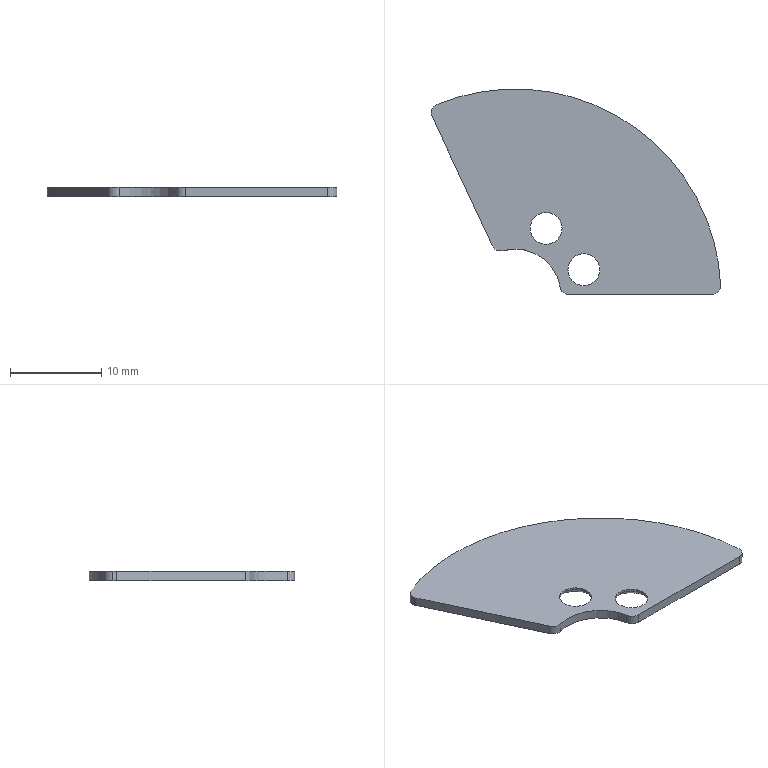Part | NX | features BREP 1 | 1 solid | 19 faces | box 31.647 x 22.5 x 1 mm | volume 455.867 mm3 | cylinder 11 | cone 4 | plane 4 | commonest cylinder face diameters 2 x5 3.5 x4 10 x1 45 x1
STEP:
#1=CARTESIAN_POINT('',(-2.5,5.362,1.));
#2=VERTEX_POINT('',#1);
#3=CARTESIAN_POINT('',(-1.328,4.82,1.));
#4=VERTEX_POINT('',#3);
#5=CARTESIAN_POINT('',(-1.594,5.784,1.));
#6=DIRECTION('',(0.,0.,1.));
#7=DIRECTION('',(1.,0.,0.));
#8=AXIS2_PLACEMENT_3D('',#5,#6,#7);
#9=CIRCLE('',#8,1.);
#10=EDGE_CURVE('',#2,#4,#9,.T.);
#11=ORIENTED_EDGE('',*,*,#10,.F.);
#12=CARTESIAN_POINT('',(-2.5,5.362,0.));
#13=VERTEX_POINT('',#12);
#14=CARTESIAN_POINT('',(-2.5,5.362,10.));
#15=DIRECTION('',(0.,0.,1.));
#16=VECTOR('',#15,1000.);
#17=LINE('',#14,#16);
#18=EDGE_CURVE('',#13,#2,#17,.T.);
#19=ORIENTED_EDGE('',*,*,#18,.F.);
#20=CARTESIAN_POINT('',(-1.328,4.82,0.));
#21=VERTEX_POINT('',#20);
#22=CARTESIAN_POINT('',(-1.594,5.784,0.));
#23=DIRECTION('',(0.,0.,-1.));
#24=DIRECTION('',(1.,0.,0.));
#25=AXIS2_PLACEMENT_3D('',#22,#23,#24);
#26=CIRCLE('',#25,1.);
#27=EDGE_CURVE('',#21,#13,#26,.T.);
#28=ORIENTED_EDGE('',*,*,#27,.F.);
#29=CARTESIAN_POINT('',(-1.328,4.82,1.));
#30=DIRECTION('',(0.,0.,-1.));
#31=VECTOR('',#30,1000.);
#32=LINE('',#29,#31);
#33=EDGE_CURVE('',#4,#21,#32,.T.);
#34=ORIENTED_EDGE('',*,*,#33,.F.);
#35=EDGE_LOOP('',(#11,#19,#28,#34));
#36=FACE_BOUND('',#35,.T.);
#37=CARTESIAN_POINT('',(-1.594,5.784,1.));
#38=DIRECTION('',(0.,0.,-1.));
#39=DIRECTION('',(-1.,0.,0.));
#40=AXIS2_PLACEMENT_3D('',#37,#38,#39);
#41=CYLINDRICAL_SURFACE('',#40,1.);
#42=ADVANCED_FACE('',(#36),#41,.T.);
#43=CARTESIAN_POINT('',(5.916,0.,0.));
#44=VERTEX_POINT('',#43);
#45=CARTESIAN_POINT('',(4.93,0.8333,0.));
#46=VERTEX_POINT('',#45);
#47=CARTESIAN_POINT('',(5.916,1.,0.));
#48=DIRECTION('',(0.,0.,-1.));
#49=DIRECTION('',(1.,0.,0.));
#50=AXIS2_PLACEMENT_3D('',#47,#48,#49);
#51=CIRCLE('',#50,1.);
#52=EDGE_CURVE('',#44,#46,#51,.T.);
#53=ORIENTED_EDGE('',*,*,#52,.F.);
#54=CARTESIAN_POINT('',(5.916,0.,1.));
#55=VERTEX_POINT('',#54);
#56=CARTESIAN_POINT('',(5.916,0.,10.));
#57=DIRECTION('',(0.,0.,-1.));
#58=VECTOR('',#57,1000.);
#59=LINE('',#56,#58);
#60=EDGE_CURVE('',#55,#44,#59,.T.);
#61=ORIENTED_EDGE('',*,*,#60,.F.);
#62=CARTESIAN_POINT('',(4.93,0.8333,1.));
#63=VERTEX_POINT('',#62);
#64=CARTESIAN_POINT('',(5.916,1.,1.));
#65=DIRECTION('',(0.,0.,1.));
#66=DIRECTION('',(1.,0.,0.));
#67=AXIS2_PLACEMENT_3D('',#64,#65,#66);
#68=CIRCLE('',#67,1.);
#69=EDGE_CURVE('',#63,#55,#68,.T.);
#70=ORIENTED_EDGE('',*,*,#69,.F.);
#71=CARTESIAN_POINT('',(4.93,0.8333,1.));
#72=DIRECTION('',(0.,0.,1.));
#73=VECTOR('',#72,1000.);
#74=LINE('',#71,#73);
#75=EDGE_CURVE('',#46,#63,#74,.T.);
#76=ORIENTED_EDGE('',*,*,#75,.F.);
#77=EDGE_LOOP('',(#53,#61,#70,#76));
#78=FACE_BOUND('',#77,.T.);
#79=CARTESIAN_POINT('',(5.916,1.,1.));
#80=DIRECTION('',(0.,0.,-1.));
#81=DIRECTION('',(-1.,0.,0.));
#82=AXIS2_PLACEMENT_3D('',#79,#80,#81);
#83=CYLINDRICAL_SURFACE('',#82,1.);
#84=ADVANCED_FACE('',(#78),#83,.T.);
#85=CARTESIAN_POINT('',(-9.17,19.887,1.));
#86=VERTEX_POINT('',#85);
#87=CARTESIAN_POINT('',(-9.17,19.887,0.));
#88=VERTEX_POINT('',#87);
#89=CARTESIAN_POINT('',(-9.17,19.887,1.));
#90=DIRECTION('',(0.,0.,-1.));
#91=VECTOR('',#90,1000.);
#92=LINE('',#89,#91);
#93=EDGE_CURVE('',#86,#88,#92,.T.);
#94=ORIENTED_EDGE('',*,*,#93,.F.);
#95=CARTESIAN_POINT('',(-8.55,20.812,1.));
#96=VERTEX_POINT('',#95);
#97=CARTESIAN_POINT('',(-8.17,19.887,1.));
#98=DIRECTION('',(0.,0.,1.));
#99=DIRECTION('',(1.,0.,0.));
#100=AXIS2_PLACEMENT_3D('',#97,#98,#99);
#101=CIRCLE('',#100,1.);
#102=EDGE_CURVE('',#96,#86,#101,.T.);
#103=ORIENTED_EDGE('',*,*,#102,.F.);
#104=CARTESIAN_POINT('',(-8.55,20.812,0.));
#105=VERTEX_POINT('',#104);
#106=CARTESIAN_POINT('',(-8.55,20.812,1.));
#107=DIRECTION('',(0.,0.,1.));
#108=VECTOR('',#107,1000.);
#109=LINE('',#106,#108);
#110=EDGE_CURVE('',#105,#96,#109,.T.);
#111=ORIENTED_EDGE('',*,*,#110,.F.);
#112=CARTESIAN_POINT('',(-8.17,19.887,0.));
#113=DIRECTION('',(0.,0.,-1.));
#114=DIRECTION('',(1.,0.,0.));
#115=AXIS2_PLACEMENT_3D('',#112,#113,#114);
#116=CIRCLE('',#115,1.);
#117=EDGE_CURVE('',#88,#105,#116,.T.);
#118=ORIENTED_EDGE('',*,*,#117,.F.);
#119=EDGE_LOOP('',(#94,#103,#111,#118));
#120=FACE_BOUND('',#119,.T.);
#121=CARTESIAN_POINT('',(-8.17,19.887,1.));
#122=DIRECTION('',(0.,0.,-1.));
#123=DIRECTION('',(-1.,0.,0.));
#124=AXIS2_PLACEMENT_3D('',#121,#122,#123);
#125=CYLINDRICAL_SURFACE('',#124,1.);
#126=ADVANCED_FACE('',(#120),#125,.T.);
#127=CARTESIAN_POINT('',(22.476,1.047,0.));
#128=VERTEX_POINT('',#127);
#129=CARTESIAN_POINT('',(21.477,0.,0.));
#130=VERTEX_POINT('',#129);
#131=CARTESIAN_POINT('',(21.477,1.,0.));
#132=DIRECTION('',(0.,0.,-1.));
#133=DIRECTION('',(1.,0.,0.));
#134=AXIS2_PLACEMENT_3D('',#131,#132,#133);
#135=CIRCLE('',#134,1.);
#136=EDGE_CURVE('',#128,#130,#135,.T.);
#137=ORIENTED_EDGE('',*,*,#136,.F.);
#138=CARTESIAN_POINT('',(22.476,1.047,1.));
#139=VERTEX_POINT('',#138);
#140=CARTESIAN_POINT('',(22.476,1.047,1.));
#141=DIRECTION('',(0.,0.,-1.));
#142=VECTOR('',#141,1000.);
#143=LINE('',#140,#142);
#144=EDGE_CURVE('',#139,#128,#143,.T.);
#145=ORIENTED_EDGE('',*,*,#144,.F.);
#146=CARTESIAN_POINT('',(21.477,0.,1.));
#147=VERTEX_POINT('',#146);
#148=CARTESIAN_POINT('',(21.477,1.,1.));
#149=DIRECTION('',(0.,0.,1.));
#150=DIRECTION('',(1.,0.,0.));
#151=AXIS2_PLACEMENT_3D('',#148,#149,#150);
#152=CIRCLE('',#151,1.);
#153=EDGE_CURVE('',#147,#139,#152,.T.);
#154=ORIENTED_EDGE('',*,*,#153,.F.);
#155=CARTESIAN_POINT('',(21.477,0.,1.));
#156=DIRECTION('',(0.,0.,1.));
#157=VECTOR('',#156,1000.);
#158=LINE('',#155,#157);
#159=EDGE_CURVE('',#130,#147,#158,.T.);
#160=ORIENTED_EDGE('',*,*,#159,.F.);
#161=EDGE_LOOP('',(#137,#145,#154,#160));
#162=FACE_BOUND('',#161,.T.);
#163=CARTESIAN_POINT('',(21.477,1.,1.));
#164=DIRECTION('',(0.,0.,-1.));
#165=DIRECTION('',(-1.,0.,0.));
#166=AXIS2_PLACEMENT_3D('',#163,#164,#165);
#167=CYLINDRICAL_SURFACE('',#166,1.);
#168=ADVANCED_FACE('',(#162),#167,.T.);
#169=CARTESIAN_POINT('',(9.268,2.736,0.75));
#170=VERTEX_POINT('',#169);
#171=CARTESIAN_POINT('',(10.018,2.736,0.));
#172=VERTEX_POINT('',#171);
#173=CARTESIAN_POINT('',(9.268,2.736,0.75));
#174=DIRECTION('',(0.7071,0.,-0.7071));
#175=VECTOR('',#174,1000.);
#176=LINE('',#173,#175);
#177=EDGE_CURVE('',#170,#172,#176,.T.);
#178=ORIENTED_EDGE('',*,*,#177,.F.);
#179=CARTESIAN_POINT('',(5.768,2.736,0.75));
#180=VERTEX_POINT('',#179);
#181=CARTESIAN_POINT('',(7.518,2.736,0.75));
#182=DIRECTION('',(0.,0.,-1.));
#183=DIRECTION('',(1.,0.,0.));
#184=AXIS2_PLACEMENT_3D('',#181,#182,#183);
#185=CIRCLE('',#184,1.75);
#186=EDGE_CURVE('',#180,#170,#185,.T.);
#187=ORIENTED_EDGE('',*,*,#186,.F.);
#188=CARTESIAN_POINT('',(5.018,2.736,0.));
#189=VERTEX_POINT('',#188);
#190=CARTESIAN_POINT('',(5.768,2.736,0.75));
#191=DIRECTION('',(-0.7071,0.,-0.7071));
#192=VECTOR('',#191,1000.);
#193=LINE('',#190,#192);
#194=EDGE_CURVE('',#180,#189,#193,.T.);
#195=ORIENTED_EDGE('',*,*,#194,.T.);
#196=CARTESIAN_POINT('',(7.518,2.736,0.));
#197=DIRECTION('',(0.,0.,1.));
#198=DIRECTION('',(1.,0.,0.));
#199=AXIS2_PLACEMENT_3D('',#196,#197,#198);
#200=CIRCLE('',#199,2.5);
#201=EDGE_CURVE('',#172,#189,#200,.T.);
#202=ORIENTED_EDGE('',*,*,#201,.F.);
#203=EDGE_LOOP('',(#178,#187,#195,#202));
#204=FACE_BOUND('',#203,.T.);
#205=CARTESIAN_POINT('',(7.518,2.736,0.75));
#206=DIRECTION('',(0.,0.,-1.));
#207=DIRECTION('',(-1.,0.,0.));
#208=AXIS2_PLACEMENT_3D('',#205,#206,#207);
#209=CONICAL_SURFACE('',#208,1.75,0.7854);
#210=ADVANCED_FACE('',(#204),#209,.F.);
#211=CARTESIAN_POINT('',(5.131,7.25,0.75));
#212=VERTEX_POINT('',#211);
#213=CARTESIAN_POINT('',(5.881,7.25,0.));
#214=VERTEX_POINT('',#213);
#215=CARTESIAN_POINT('',(5.131,7.25,0.75));
#216=DIRECTION('',(0.7071,0.,-0.7071));
#217=VECTOR('',#216,1000.);
#218=LINE('',#215,#217);
#219=EDGE_CURVE('',#212,#214,#218,.T.);
#220=ORIENTED_EDGE('',*,*,#219,.F.);
#221=CARTESIAN_POINT('',(1.631,7.25,0.75));
#222=VERTEX_POINT('',#221);
#223=CARTESIAN_POINT('',(3.381,7.25,0.75));
#224=DIRECTION('',(0.,0.,-1.));
#225=DIRECTION('',(1.,0.,0.));
#226=AXIS2_PLACEMENT_3D('',#223,#224,#225);
#227=CIRCLE('',#226,1.75);
#228=EDGE_CURVE('',#222,#212,#227,.T.);
#229=ORIENTED_EDGE('',*,*,#228,.F.);
#230=CARTESIAN_POINT('',(0.8809,7.25,0.));
#231=VERTEX_POINT('',#230);
#232=CARTESIAN_POINT('',(1.631,7.25,0.75));
#233=DIRECTION('',(-0.7071,0.,-0.7071));
#234=VECTOR('',#233,1000.);
#235=LINE('',#232,#234);
#236=EDGE_CURVE('',#222,#231,#235,.T.);
#237=ORIENTED_EDGE('',*,*,#236,.T.);
#238=CARTESIAN_POINT('',(3.381,7.25,0.));
#239=DIRECTION('',(0.,0.,1.));
#240=DIRECTION('',(1.,0.,0.));
#241=AXIS2_PLACEMENT_3D('',#238,#239,#240);
#242=CIRCLE('',#241,2.5);
#243=EDGE_CURVE('',#214,#231,#242,.T.);
#244=ORIENTED_EDGE('',*,*,#243,.F.);
#245=EDGE_LOOP('',(#220,#229,#237,#244));
#246=FACE_BOUND('',#245,.T.);
#247=CARTESIAN_POINT('',(3.381,7.25,0.75));
#248=DIRECTION('',(0.,0.,-1.));
#249=DIRECTION('',(-1.,0.,0.));
#250=AXIS2_PLACEMENT_3D('',#247,#248,#249);
#251=CONICAL_SURFACE('',#250,1.75,0.7854);
#252=ADVANCED_FACE('',(#246),#251,.F.);
#253=CARTESIAN_POINT('',(9.268,2.736,1.));
#254=VERTEX_POINT('',#253);
#255=CARTESIAN_POINT('',(9.268,2.736,10.));
#256=DIRECTION('',(0.,0.,-1.));
#257=VECTOR('',#256,1000.);
#258=LINE('',#255,#257);
#259=EDGE_CURVE('',#254,#170,#258,.T.);
#260=ORIENTED_EDGE('',*,*,#259,.F.);
#261=CARTESIAN_POINT('',(5.768,2.736,1.));
#262=VERTEX_POINT('',#261);
#263=CARTESIAN_POINT('',(7.518,2.736,1.));
#264=DIRECTION('',(0.,0.,1.));
#265=DIRECTION('',(1.,0.,0.));
#266=AXIS2_PLACEMENT_3D('',#263,#264,#265);
#267=CIRCLE('',#266,1.75);
#268=EDGE_CURVE('',#254,#262,#267,.T.);
#269=ORIENTED_EDGE('',*,*,#268,.T.);
#270=CARTESIAN_POINT('',(5.768,2.736,10.));
#271=DIRECTION('',(0.,0.,-1.));
#272=VECTOR('',#271,1000.);
#273=LINE('',#270,#272);
#274=EDGE_CURVE('',#262,#180,#273,.T.);
#275=ORIENTED_EDGE('',*,*,#274,.T.);
#276=ORIENTED_EDGE('',*,*,#186,.T.);
#277=EDGE_LOOP('',(#260,#269,#275,#276));
#278=FACE_BOUND('',#277,.T.);
#279=CARTESIAN_POINT('',(7.518,2.736,10.));
#280=DIRECTION('',(0.,0.,-1.));
#281=DIRECTION('',(-1.,0.,0.));
#282=AXIS2_PLACEMENT_3D('',#279,#280,#281);
#283=CYLINDRICAL_SURFACE('',#282,1.75);
#284=ADVANCED_FACE('',(#278),#283,.F.);
#285=CARTESIAN_POINT('',(5.131,7.25,1.));
#286=VERTEX_POINT('',#285);
#287=CARTESIAN_POINT('',(5.131,7.25,10.));
#288=DIRECTION('',(0.,0.,-1.));
#289=VECTOR('',#288,1000.);
#290=LINE('',#287,#289);
#291=EDGE_CURVE('',#286,#212,#290,.T.);
#292=ORIENTED_EDGE('',*,*,#291,.F.);
#293=CARTESIAN_POINT('',(1.631,7.25,1.));
#294=VERTEX_POINT('',#293);
#295=CARTESIAN_POINT('',(3.381,7.25,1.));
#296=DIRECTION('',(0.,0.,1.));
#297=DIRECTION('',(1.,0.,0.));
#298=AXIS2_PLACEMENT_3D('',#295,#296,#297);
#299=CIRCLE('',#298,1.75);
#300=EDGE_CURVE('',#286,#294,#299,.T.);
#301=ORIENTED_EDGE('',*,*,#300,.T.);
#302=CARTESIAN_POINT('',(1.631,7.25,10.));
#303=DIRECTION('',(0.,0.,-1.));
#304=VECTOR('',#303,1000.);
#305=LINE('',#302,#304);
#306=EDGE_CURVE('',#294,#222,#305,.T.);
#307=ORIENTED_EDGE('',*,*,#306,.T.);
#308=ORIENTED_EDGE('',*,*,#228,.T.);
#309=EDGE_LOOP('',(#292,#301,#307,#308));
#310=FACE_BOUND('',#309,.T.);
#311=CARTESIAN_POINT('',(3.381,7.25,10.));
#312=DIRECTION('',(0.,0.,-1.));
#313=DIRECTION('',(-1.,0.,0.));
#314=AXIS2_PLACEMENT_3D('',#311,#312,#313);
#315=CYLINDRICAL_SURFACE('',#314,1.75);
#316=ADVANCED_FACE('',(#310),#315,.F.);
#317=CARTESIAN_POINT('',(-9.076,19.465,1.));
#318=VERTEX_POINT('',#317);
#319=CARTESIAN_POINT('',(0.,0.,1.));
#320=DIRECTION('',(0.4226,-0.9063,0.));
#321=VECTOR('',#320,1000.);
#322=LINE('',#319,#321);
#323=EDGE_CURVE('',#318,#2,#322,.T.);
#324=ORIENTED_EDGE('',*,*,#323,.F.);
#325=CARTESIAN_POINT('',(-9.076,19.465,0.));
#326=VERTEX_POINT('',#325);
#327=CARTESIAN_POINT('',(-9.076,19.465,0.));
#328=DIRECTION('',(0.,0.,-1.));
#329=VECTOR('',#328,1000.);
#330=LINE('',#327,#329);
#331=EDGE_CURVE('',#318,#326,#330,.T.);
#332=ORIENTED_EDGE('',*,*,#331,.T.);
#333=CARTESIAN_POINT('',(0.,0.,0.));
#334=DIRECTION('',(-0.4226,0.9063,0.));
#335=VECTOR('',#334,1000.);
#336=LINE('',#333,#335);
#337=EDGE_CURVE('',#13,#326,#336,.T.);
#338=ORIENTED_EDGE('',*,*,#337,.F.);
#339=ORIENTED_EDGE('',*,*,#18,.T.);
#340=EDGE_LOOP('',(#324,#332,#338,#339));
#341=FACE_BOUND('',#340,.T.);
#342=CARTESIAN_POINT('',(0.,0.,10.));
#343=DIRECTION('',(-0.9063,-0.4226,0.));
#344=DIRECTION('',(0.4226,-0.9063,0.));
#345=AXIS2_PLACEMENT_3D('',#342,#343,#344);
#346=PLANE('',#345);
#347=ADVANCED_FACE('',(#341),#346,.T.);
#348=CARTESIAN_POINT('',(0.,0.,0.));
#349=DIRECTION('',(-1.,0.,0.));
#350=VECTOR('',#349,1000.);
#351=LINE('',#348,#350);
#352=EDGE_CURVE('',#130,#44,#351,.T.);
#353=ORIENTED_EDGE('',*,*,#352,.F.);
#354=ORIENTED_EDGE('',*,*,#159,.T.);
#355=CARTESIAN_POINT('',(0.,0.,1.));
#356=DIRECTION('',(1.,0.,0.));
#357=VECTOR('',#356,1000.);
#358=LINE('',#355,#357);
#359=EDGE_CURVE('',#55,#147,#358,.T.);
#360=ORIENTED_EDGE('',*,*,#359,.F.);
#361=ORIENTED_EDGE('',*,*,#60,.T.);
#362=EDGE_LOOP('',(#353,#354,#360,#361));
#363=FACE_BOUND('',#362,.T.);
#364=CARTESIAN_POINT('',(0.,0.,10.));
#365=DIRECTION('',(0.,-1.,0.));
#366=DIRECTION('',(0.,0.,-1.));
#367=AXIS2_PLACEMENT_3D('',#364,#365,#366);
#368=PLANE('',#367);
#369=ADVANCED_FACE('',(#363),#368,.T.);
#370=CARTESIAN_POINT('',(0.,0.,0.));
#371=DIRECTION('',(0.,0.,1.));
#372=DIRECTION('',(1.,0.,0.));
#373=AXIS2_PLACEMENT_3D('',#370,#371,#372);
#374=CIRCLE('',#373,5.);
#375=EDGE_CURVE('',#46,#21,#374,.T.);
#376=ORIENTED_EDGE('',*,*,#375,.F.);
#377=ORIENTED_EDGE('',*,*,#75,.T.);
#378=CARTESIAN_POINT('',(0.,0.,1.));
#379=DIRECTION('',(0.,0.,1.));
#380=DIRECTION('',(1.,0.,0.));
#381=AXIS2_PLACEMENT_3D('',#378,#379,#380);
#382=CIRCLE('',#381,5.);
#383=EDGE_CURVE('',#63,#4,#382,.T.);
#384=ORIENTED_EDGE('',*,*,#383,.T.);
#385=ORIENTED_EDGE('',*,*,#33,.T.);
#386=EDGE_LOOP('',(#376,#377,#384,#385));
#387=FACE_BOUND('',#386,.T.);
#388=CARTESIAN_POINT('',(0.,0.,1.));
#389=DIRECTION('',(0.,0.,-1.));
#390=DIRECTION('',(-1.,0.,0.));
#391=AXIS2_PLACEMENT_3D('',#388,#389,#390);
#392=CYLINDRICAL_SURFACE('',#391,5.);
#393=ADVANCED_FACE('',(#387),#392,.F.);
#394=CARTESIAN_POINT('',(0.,0.,1.));
#395=DIRECTION('',(0.,0.,1.));
#396=DIRECTION('',(1.,0.,0.));
#397=AXIS2_PLACEMENT_3D('',#394,#395,#396);
#398=CIRCLE('',#397,22.5);
#399=EDGE_CURVE('',#139,#96,#398,.T.);
#400=ORIENTED_EDGE('',*,*,#399,.F.);
#401=ORIENTED_EDGE('',*,*,#144,.T.);
#402=CARTESIAN_POINT('',(0.,0.,0.));
#403=DIRECTION('',(0.,0.,1.));
#404=DIRECTION('',(1.,0.,0.));
#405=AXIS2_PLACEMENT_3D('',#402,#403,#404);
#406=CIRCLE('',#405,22.5);
#407=EDGE_CURVE('',#128,#105,#406,.T.);
#408=ORIENTED_EDGE('',*,*,#407,.T.);
#409=ORIENTED_EDGE('',*,*,#110,.T.);
#410=EDGE_LOOP('',(#400,#401,#408,#409));
#411=FACE_BOUND('',#410,.T.);
#412=CARTESIAN_POINT('',(0.,0.,1.));
#413=DIRECTION('',(0.,0.,-1.));
#414=DIRECTION('',(-1.,0.,0.));
#415=AXIS2_PLACEMENT_3D('',#412,#413,#414);
#416=CYLINDRICAL_SURFACE('',#415,22.5);
#417=ADVANCED_FACE('',(#411),#416,.T.);
#418=ORIENTED_EDGE('',*,*,#407,.F.);
#419=ORIENTED_EDGE('',*,*,#136,.T.);
#420=ORIENTED_EDGE('',*,*,#352,.T.);
#421=ORIENTED_EDGE('',*,*,#52,.T.);
#422=ORIENTED_EDGE('',*,*,#375,.T.);
#423=ORIENTED_EDGE('',*,*,#27,.T.);
#424=ORIENTED_EDGE('',*,*,#337,.T.);
#425=CARTESIAN_POINT('',(-8.17,19.887,0.));
#426=DIRECTION('',(0.,0.,-1.));
#427=DIRECTION('',(1.,0.,0.));
#428=AXIS2_PLACEMENT_3D('',#425,#426,#427);
#429=CIRCLE('',#428,1.);
#430=EDGE_CURVE('',#326,#88,#429,.T.);
#431=ORIENTED_EDGE('',*,*,#430,.T.);
#432=ORIENTED_EDGE('',*,*,#117,.T.);
#433=EDGE_LOOP('',(#418,#419,#420,#421,#422,#423,#424,#431,#432));
#434=FACE_BOUND('',#433,.T.);
#435=CARTESIAN_POINT('',(7.518,2.736,0.));
#436=DIRECTION('',(0.,0.,1.));
#437=DIRECTION('',(1.,0.,0.));
#438=AXIS2_PLACEMENT_3D('',#435,#436,#437);
#439=CIRCLE('',#438,2.5);
#440=EDGE_CURVE('',#189,#172,#439,.T.);
#441=ORIENTED_EDGE('',*,*,#440,.T.);
#442=ORIENTED_EDGE('',*,*,#201,.T.);
#443=EDGE_LOOP('',(#441,#442));
#444=FACE_BOUND('',#443,.T.);
#445=CARTESIAN_POINT('',(3.381,7.25,0.));
#446=DIRECTION('',(0.,0.,1.));
#447=DIRECTION('',(1.,0.,0.));
#448=AXIS2_PLACEMENT_3D('',#445,#446,#447);
#449=CIRCLE('',#448,2.5);
#450=EDGE_CURVE('',#231,#214,#449,.T.);
#451=ORIENTED_EDGE('',*,*,#450,.T.);
#452=ORIENTED_EDGE('',*,*,#243,.T.);
#453=EDGE_LOOP('',(#451,#452));
#454=FACE_BOUND('',#453,.T.);
#455=CARTESIAN_POINT('',(0.,0.,0.));
#456=DIRECTION('',(0.,0.,1.));
#457=DIRECTION('',(1.,0.,0.));
#458=AXIS2_PLACEMENT_3D('',#455,#456,#457);
#459=PLANE('',#458);
#460=ADVANCED_FACE('',(#434,#444,#454),#459,.F.);
#461=ORIENTED_EDGE('',*,*,#359,.T.);
#462=ORIENTED_EDGE('',*,*,#153,.T.);
#463=ORIENTED_EDGE('',*,*,#399,.T.);
#464=ORIENTED_EDGE('',*,*,#102,.T.);
#465=CARTESIAN_POINT('',(-8.17,19.887,1.));
#466=DIRECTION('',(0.,0.,1.));
#467=DIRECTION('',(1.,0.,0.));
#468=AXIS2_PLACEMENT_3D('',#465,#466,#467);
#469=CIRCLE('',#468,1.);
#470=EDGE_CURVE('',#86,#318,#469,.T.);
#471=ORIENTED_EDGE('',*,*,#470,.T.);
#472=ORIENTED_EDGE('',*,*,#323,.T.);
#473=ORIENTED_EDGE('',*,*,#10,.T.);
#474=ORIENTED_EDGE('',*,*,#383,.F.);
#475=ORIENTED_EDGE('',*,*,#69,.T.);
#476=EDGE_LOOP('',(#461,#462,#463,#464,#471,#472,#473,#474,#475));
#477=FACE_BOUND('',#476,.T.);
#478=CARTESIAN_POINT('',(3.381,7.25,1.));
#479=DIRECTION('',(0.,0.,1.));
#480=DIRECTION('',(1.,0.,0.));
#481=AXIS2_PLACEMENT_3D('',#478,#479,#480);
#482=CIRCLE('',#481,1.75);
#483=EDGE_CURVE('',#294,#286,#482,.T.);
#484=ORIENTED_EDGE('',*,*,#483,.F.);
#485=ORIENTED_EDGE('',*,*,#300,.F.);
#486=EDGE_LOOP('',(#484,#485));
#487=FACE_BOUND('',#486,.T.);
#488=CARTESIAN_POINT('',(7.518,2.736,1.));
#489=DIRECTION('',(0.,0.,1.));
#490=DIRECTION('',(1.,0.,0.));
#491=AXIS2_PLACEMENT_3D('',#488,#489,#490);
#492=CIRCLE('',#491,1.75);
#493=EDGE_CURVE('',#262,#254,#492,.T.);
#494=ORIENTED_EDGE('',*,*,#493,.F.);
#495=ORIENTED_EDGE('',*,*,#268,.F.);
#496=EDGE_LOOP('',(#494,#495));
#497=FACE_BOUND('',#496,.T.);
#498=CARTESIAN_POINT('',(0.,0.,1.));
#499=DIRECTION('',(0.,0.,1.));
#500=DIRECTION('',(1.,0.,0.));
#501=AXIS2_PLACEMENT_3D('',#498,#499,#500);
#502=PLANE('',#501);
#503=ADVANCED_FACE('',(#477,#487,#497),#502,.T.);
#504=ORIENTED_EDGE('',*,*,#483,.T.);
#505=ORIENTED_EDGE('',*,*,#291,.T.);
#506=CARTESIAN_POINT('',(3.381,7.25,0.75));
#507=DIRECTION('',(0.,0.,-1.));
#508=DIRECTION('',(1.,0.,0.));
#509=AXIS2_PLACEMENT_3D('',#506,#507,#508);
#510=CIRCLE('',#509,1.75);
#511=EDGE_CURVE('',#212,#222,#510,.T.);
#512=ORIENTED_EDGE('',*,*,#511,.T.);
#513=ORIENTED_EDGE('',*,*,#306,.F.);
#514=EDGE_LOOP('',(#504,#505,#512,#513));
#515=FACE_BOUND('',#514,.T.);
#516=CARTESIAN_POINT('',(3.381,7.25,10.));
#517=DIRECTION('',(0.,0.,-1.));
#518=DIRECTION('',(-1.,0.,0.));
#519=AXIS2_PLACEMENT_3D('',#516,#517,#518);
#520=CYLINDRICAL_SURFACE('',#519,1.75);
#521=ADVANCED_FACE('',(#515),#520,.F.);
#522=ORIENTED_EDGE('',*,*,#493,.T.);
#523=ORIENTED_EDGE('',*,*,#259,.T.);
#524=CARTESIAN_POINT('',(7.518,2.736,0.75));
#525=DIRECTION('',(0.,0.,-1.));
#526=DIRECTION('',(1.,0.,0.));
#527=AXIS2_PLACEMENT_3D('',#524,#525,#526);
#528=CIRCLE('',#527,1.75);
#529=EDGE_CURVE('',#170,#180,#528,.T.);
#530=ORIENTED_EDGE('',*,*,#529,.T.);
#531=ORIENTED_EDGE('',*,*,#274,.F.);
#532=EDGE_LOOP('',(#522,#523,#530,#531));
#533=FACE_BOUND('',#532,.T.);
#534=CARTESIAN_POINT('',(7.518,2.736,10.));
#535=DIRECTION('',(0.,0.,-1.));
#536=DIRECTION('',(-1.,0.,0.));
#537=AXIS2_PLACEMENT_3D('',#534,#535,#536);
#538=CYLINDRICAL_SURFACE('',#537,1.75);
#539=ADVANCED_FACE('',(#533),#538,.F.);
#540=ORIENTED_EDGE('',*,*,#511,.F.);
#541=ORIENTED_EDGE('',*,*,#219,.T.);
#542=ORIENTED_EDGE('',*,*,#450,.F.);
#543=ORIENTED_EDGE('',*,*,#236,.F.);
#544=EDGE_LOOP('',(#540,#541,#542,#543));
#545=FACE_BOUND('',#544,.T.);
#546=CARTESIAN_POINT('',(3.381,7.25,0.75));
#547=DIRECTION('',(0.,0.,-1.));
#548=DIRECTION('',(-1.,0.,0.));
#549=AXIS2_PLACEMENT_3D('',#546,#547,#548);
#550=CONICAL_SURFACE('',#549,1.75,0.7854);
#551=ADVANCED_FACE('',(#545),#550,.F.);
#552=ORIENTED_EDGE('',*,*,#529,.F.);
#553=ORIENTED_EDGE('',*,*,#177,.T.);
#554=ORIENTED_EDGE('',*,*,#440,.F.);
#555=ORIENTED_EDGE('',*,*,#194,.F.);
#556=EDGE_LOOP('',(#552,#553,#554,#555));
#557=FACE_BOUND('',#556,.T.);
#558=CARTESIAN_POINT('',(7.518,2.736,0.75));
#559=DIRECTION('',(0.,0.,-1.));
#560=DIRECTION('',(-1.,0.,0.));
#561=AXIS2_PLACEMENT_3D('',#558,#559,#560);
#562=CONICAL_SURFACE('',#561,1.75,0.7854);
#563=ADVANCED_FACE('',(#557),#562,.F.);
#564=ORIENTED_EDGE('',*,*,#470,.F.);
#565=ORIENTED_EDGE('',*,*,#93,.T.);
#566=ORIENTED_EDGE('',*,*,#430,.F.);
#567=ORIENTED_EDGE('',*,*,#331,.F.);
#568=EDGE_LOOP('',(#564,#565,#566,#567));
#569=FACE_BOUND('',#568,.T.);
#570=CARTESIAN_POINT('',(-8.17,19.887,1.));
#571=DIRECTION('',(0.,0.,-1.));
#572=DIRECTION('',(-1.,0.,0.));
#573=AXIS2_PLACEMENT_3D('',#570,#571,#572);
#574=CYLINDRICAL_SURFACE('',#573,1.);
#575=ADVANCED_FACE('',(#569),#574,.T.);
#576=CLOSED_SHELL('',(#42,#84,#126,#168,#210,#252,#284,#316,#347,#369,#393,#417,#460,#503,#521,#539,#551,#563,#575));
#577=MANIFOLD_SOLID_BREP('',#576);
#578=(LENGTH_UNIT()NAMED_UNIT(*)SI_UNIT(.MILLI.,.METRE.));
#579=UNCERTAINTY_MEASURE_WITH_UNIT(LENGTH_MEASURE(0.00001),#578,'','');
#580=(NAMED_UNIT(*)PLANE_ANGLE_UNIT()SI_UNIT($,.RADIAN.));
#581=(NAMED_UNIT(*)SI_UNIT($,.STERADIAN.)SOLID_ANGLE_UNIT());
#582=(GEOMETRIC_REPRESENTATION_CONTEXT(3)GLOBAL_UNCERTAINTY_ASSIGNED_CONTEXT((#579))GLOBAL_UNIT_ASSIGNED_CONTEXT((#578,#580,#581))REPRESENTATION_CONTEXT('',''));
#583=ADVANCED_BREP_SHAPE_REPRESENTATION('',(#577),#582);